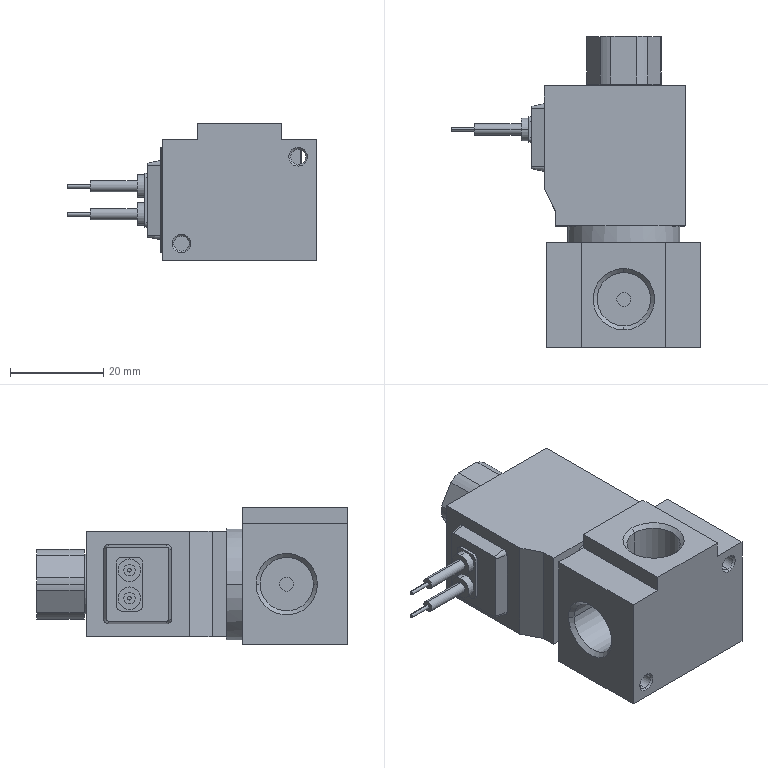Part | 1 solid | 121 faces | box 53.5 x 66.6 x 29.5 mm | volume 41442 mm3 | plane 55 | cylinder 52 | cone 14 | commonest cylinder face diameters 16 x7 3 x6 11.445 x6 0.8 x4 2 x4 2.4 x4